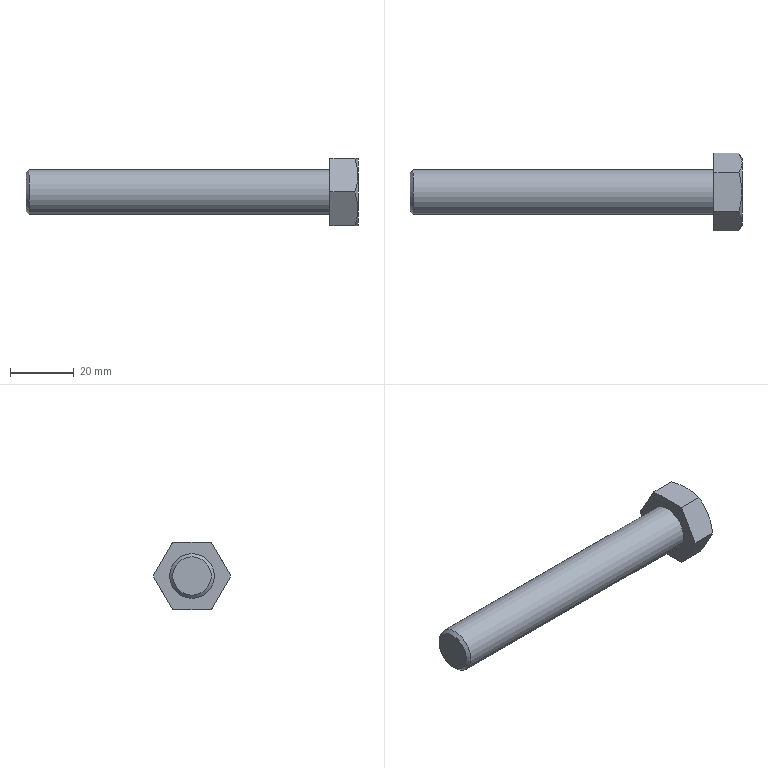Part | STEP file | 8901-M14 (bolt M14×95) | 1 solid | 12 faces | box 103.8 x 24.249 x 21 mm | volume 17952 mm3 | plane 9 | cone 2 | cylinder 1 | commonest cylinder face diameters 14 x1
STEP:
#1=CARTESIAN_POINT('',(0.,0.,0.));
#2=DIRECTION('',(0.,0.,1.));
#3=DIRECTION('',(1.,0.,0.));
#4=AXIS2_PLACEMENT_3D('',#1,#2,#3);
#5=CARTESIAN_POINT('',(1501.5,0.00003081,-188.));
#6=VERTEX_POINT('',#5);
#7=CARTESIAN_POINT('',(1501.5,0.00003081,-195.));
#8=DIRECTION('',(1.,0.,0.));
#9=DIRECTION('',(0.,0.,1.));
#10=AXIS2_PLACEMENT_3D('',#7,#8,#9);
#11=CIRCLE('',#10,7.);
#12=CARTESIAN_POINT('',(1501.5,0.00003081,-195.));
#13=DIRECTION('',(1.,0.,0.));
#14=DIRECTION('',(0.,0.,1.));
#15=AXIS2_PLACEMENT_3D('',#12,#13,#14);
#16=CONICAL_SURFACE('',#15,7.,0.7854);
#17=CARTESIAN_POINT('',(0.,0.));
#18=DIRECTION('',(1.,0.));
#19=VECTOR('',#18,1.);
#20=LINE('',#17,#19);
#21=(GEOMETRIC_REPRESENTATION_CONTEXT(2)PARAMETRIC_REPRESENTATION_CONTEXT()REPRESENTATION_CONTEXT('',''));
#22=DEFINITIONAL_REPRESENTATION('',(#20),#21);
#23=PCURVE('',#16,#22);
#24=CARTESIAN_POINT('',(1595.5,0.00003081,-195.));
#25=DIRECTION('',(-1.,0.,0.));
#26=DIRECTION('',(0.,0.,-1.));
#27=AXIS2_PLACEMENT_3D('',#24,#25,#26);
#28=CYLINDRICAL_SURFACE('',#27,7.);
#29=CARTESIAN_POINT('',(9.425,94.));
#30=DIRECTION('',(-1.,0.));
#31=VECTOR('',#30,1.);
#32=LINE('',#29,#31);
#33=(GEOMETRIC_REPRESENTATION_CONTEXT(2)PARAMETRIC_REPRESENTATION_CONTEXT()REPRESENTATION_CONTEXT('',''));
#34=DEFINITIONAL_REPRESENTATION('',(#32),#33);
#35=PCURVE('',#28,#34);
#36=SURFACE_CURVE('',#11,(#23,#35),.PCURVE_S1.);
#37=EDGE_CURVE('',#6,#6,#36,.T.);
#38=ORIENTED_EDGE('',*,*,#37,.F.);
#39=CARTESIAN_POINT('',(1500.5,0.00003081,-189.));
#40=VERTEX_POINT('',#39);
#41=CARTESIAN_POINT('',(1500.5,0.00003081,-189.));
#42=CARTESIAN_POINT('',(1501.5,0.00003081,-188.));
#43=B_SPLINE_CURVE_WITH_KNOTS('',1,(#41,#42),.UNSPECIFIED.,.F.,.F.,(2,2),(-1.414,0.),.PIECEWISE_BEZIER_KNOTS.);
#44=CARTESIAN_POINT('',(0.,0.));
#45=DIRECTION('',(0.,1.));
#46=VECTOR('',#45,1.);
#47=LINE('',#44,#46);
#48=(GEOMETRIC_REPRESENTATION_CONTEXT(2)PARAMETRIC_REPRESENTATION_CONTEXT()REPRESENTATION_CONTEXT('',''));
#49=DEFINITIONAL_REPRESENTATION('',(#47),#48);
#50=PCURVE('',#16,#49);
#51=CARTESIAN_POINT('',(6.283,0.));
#52=DIRECTION('',(0.,1.));
#53=VECTOR('',#52,1.);
#54=LINE('',#51,#53);
#55=(GEOMETRIC_REPRESENTATION_CONTEXT(2)PARAMETRIC_REPRESENTATION_CONTEXT()REPRESENTATION_CONTEXT('',''));
#56=DEFINITIONAL_REPRESENTATION('',(#54),#55);
#57=PCURVE('',#16,#56);
#58=SEAM_CURVE('',#43,(#50,#57),.PCURVE_S1.);
#59=EDGE_CURVE('',#40,#6,#58,.T.);
#60=ORIENTED_EDGE('',*,*,#59,.F.);
#61=CARTESIAN_POINT('',(1500.5,0.00003081,-195.));
#62=DIRECTION('',(-1.,0.,0.));
#63=DIRECTION('',(0.,0.,1.));
#64=AXIS2_PLACEMENT_3D('',#61,#62,#63);
#65=CIRCLE('',#64,6.);
#66=CARTESIAN_POINT('',(6.283,-1.));
#67=DIRECTION('',(-1.,0.));
#68=VECTOR('',#67,1.);
#69=LINE('',#66,#68);
#70=(GEOMETRIC_REPRESENTATION_CONTEXT(2)PARAMETRIC_REPRESENTATION_CONTEXT()REPRESENTATION_CONTEXT('',''));
#71=DEFINITIONAL_REPRESENTATION('',(#69),#70);
#72=PCURVE('',#16,#71);
#73=CARTESIAN_POINT('',(1500.5,0.00003081,-195.));
#74=DIRECTION('',(-1.,0.,0.));
#75=DIRECTION('',(0.,0.,-1.));
#76=AXIS2_PLACEMENT_3D('',#73,#74,#75);
#77=PLANE('',#76);
#78=CARTESIAN_POINT('',(0.,0.));
#79=DIRECTION('',(-1.,0.));
#80=AXIS2_PLACEMENT_2D('',#78,#79);
#81=CIRCLE('',#80,6.);
#82=(GEOMETRIC_REPRESENTATION_CONTEXT(2)PARAMETRIC_REPRESENTATION_CONTEXT()REPRESENTATION_CONTEXT('',''));
#83=DEFINITIONAL_REPRESENTATION('',(#81),#82);
#84=PCURVE('',#77,#83);
#85=SURFACE_CURVE('',#65,(#72,#84),.PCURVE_S1.);
#86=EDGE_CURVE('',#40,#40,#85,.T.);
#87=ORIENTED_EDGE('',*,*,#86,.F.);
#88=ORIENTED_EDGE('',*,*,#59,.T.);
#89=EDGE_LOOP('',(#38,#60,#87,#88));
#90=FACE_BOUND('',#89,.T.);
#91=ADVANCED_FACE('',(#90),#16,.T.);
#92=ORIENTED_EDGE('',*,*,#86,.T.);
#93=EDGE_LOOP('',(#92));
#94=FACE_BOUND('',#93,.T.);
#95=ADVANCED_FACE('',(#94),#77,.T.);
#96=CARTESIAN_POINT('',(1604.3,0.00003081,-205.395));
#97=VERTEX_POINT('',#96);
#98=CARTESIAN_POINT('',(1604.3,0.00003081,-195.));
#99=DIRECTION('',(1.,0.,0.));
#100=DIRECTION('',(0.,0.,-1.));
#101=AXIS2_PLACEMENT_3D('',#98,#99,#100);
#102=CIRCLE('',#101,10.395);
#103=CARTESIAN_POINT('',(1604.3,0.00003081,-195.));
#104=DIRECTION('',(1.,0.,0.));
#105=DIRECTION('',(0.,0.,1.));
#106=AXIS2_PLACEMENT_3D('',#103,#104,#105);
#107=PLANE('',#106);
#108=CARTESIAN_POINT('',(0.,0.));
#109=DIRECTION('',(-1.,0.));
#110=AXIS2_PLACEMENT_2D('',#108,#109);
#111=CIRCLE('',#110,10.395);
#112=(GEOMETRIC_REPRESENTATION_CONTEXT(2)PARAMETRIC_REPRESENTATION_CONTEXT()REPRESENTATION_CONTEXT('',''));
#113=DEFINITIONAL_REPRESENTATION('',(#111),#112);
#114=PCURVE('',#107,#113);
#115=CARTESIAN_POINT('',(1610.302,0.00003081,-195.));
#116=DIRECTION('',(-1.,0.,0.));
#117=DIRECTION('',(0.,0.,-1.));
#118=AXIS2_PLACEMENT_3D('',#115,#116,#117);
#119=CONICAL_SURFACE('',#118,0.,1.047);
#120=CARTESIAN_POINT('',(6.283,6.002));
#121=DIRECTION('',(-1.,0.));
#122=VECTOR('',#121,1.);
#123=LINE('',#120,#122);
#124=(GEOMETRIC_REPRESENTATION_CONTEXT(2)PARAMETRIC_REPRESENTATION_CONTEXT()REPRESENTATION_CONTEXT('',''));
#125=DEFINITIONAL_REPRESENTATION('',(#123),#124);
#126=PCURVE('',#119,#125);
#127=SURFACE_CURVE('',#102,(#114,#126),.PCURVE_S1.);
#128=EDGE_CURVE('',#97,#97,#127,.T.);
#129=ORIENTED_EDGE('',*,*,#128,.T.);
#130=EDGE_LOOP('',(#129));
#131=FACE_BOUND('',#130,.T.);
#132=ADVANCED_FACE('',(#131),#107,.T.);
#133=ORIENTED_EDGE('',*,*,#128,.F.);
#134=CARTESIAN_POINT('',(1604.239,0.00003081,-205.5));
#135=VERTEX_POINT('',#134);
#136=CARTESIAN_POINT('',(1604.3,0.00003081,-205.395));
#137=CARTESIAN_POINT('',(1604.239,0.00003081,-205.5));
#138=B_SPLINE_CURVE_WITH_KNOTS('',1,(#136,#137),.UNSPECIFIED.,.F.,.F.,(2,2),(12.003,12.124),.PIECEWISE_BEZIER_KNOTS.);
#139=CARTESIAN_POINT('',(6.283,0.));
#140=DIRECTION('',(0.,1.));
#141=VECTOR('',#140,1.);
#142=LINE('',#139,#141);
#143=(GEOMETRIC_REPRESENTATION_CONTEXT(2)PARAMETRIC_REPRESENTATION_CONTEXT()REPRESENTATION_CONTEXT('',''));
#144=DEFINITIONAL_REPRESENTATION('',(#142),#143);
#145=PCURVE('',#119,#144);
#146=CARTESIAN_POINT('',(0.,0.));
#147=DIRECTION('',(0.,1.));
#148=VECTOR('',#147,1.);
#149=LINE('',#146,#148);
#150=(GEOMETRIC_REPRESENTATION_CONTEXT(2)PARAMETRIC_REPRESENTATION_CONTEXT()REPRESENTATION_CONTEXT('',''));
#151=DEFINITIONAL_REPRESENTATION('',(#149),#150);
#152=PCURVE('',#119,#151);
#153=SEAM_CURVE('',#138,(#145,#152),.PCURVE_S1.);
#154=EDGE_CURVE('',#97,#135,#153,.T.);
#155=ORIENTED_EDGE('',*,*,#154,.T.);
#156=CARTESIAN_POINT('',(1603.302,6.062,-205.5));
#157=VERTEX_POINT('',#156);
#158=CARTESIAN_POINT('',(1603.302,6.062,-205.5));
#159=CARTESIAN_POINT('',(1603.873,4.083,-205.5));
#160=CARTESIAN_POINT('',(1604.238,2.073,-205.5));
#161=CARTESIAN_POINT('',(1604.241,-2.05,-205.5));
#162=CARTESIAN_POINT('',(1603.874,-4.08,-205.5));
#163=CARTESIAN_POINT('',(1603.302,-6.062,-205.5));
#164=B_SPLINE_CURVE_WITH_KNOTS('',3,(#158,#159,#160,#161,#162,#163),.UNSPECIFIED.,.F.,.F.,(4,2,4),(0.,0.5,1.),.UNSPECIFIED.);
#165=CARTESIAN_POINT('',(5.76,7.));
#166=CARTESIAN_POINT('',(5.772,6.948));
#167=CARTESIAN_POINT('',(5.799,6.847));
#168=CARTESIAN_POINT('',(5.84,6.707));
#169=CARTESIAN_POINT('',(5.883,6.579));
#170=CARTESIAN_POINT('',(5.928,6.463));
#171=CARTESIAN_POINT('',(5.975,6.36));
#172=CARTESIAN_POINT('',(6.023,6.271));
#173=CARTESIAN_POINT('',(6.073,6.197));
#174=CARTESIAN_POINT('',(6.124,6.138));
#175=CARTESIAN_POINT('',(6.176,6.095));
#176=CARTESIAN_POINT('',(6.229,6.068));
#177=CARTESIAN_POINT('',(6.282,6.059));
#178=CARTESIAN_POINT('',(6.336,6.068));
#179=CARTESIAN_POINT('',(6.389,6.093));
#180=CARTESIAN_POINT('',(6.441,6.136));
#181=CARTESIAN_POINT('',(6.492,6.195));
#182=CARTESIAN_POINT('',(6.542,6.269));
#183=CARTESIAN_POINT('',(6.591,6.358));
#184=CARTESIAN_POINT('',(6.638,6.461));
#185=CARTESIAN_POINT('',(6.683,6.578));
#186=CARTESIAN_POINT('',(6.726,6.707));
#187=CARTESIAN_POINT('',(6.768,6.847));
#188=CARTESIAN_POINT('',(6.794,6.948));
#189=CARTESIAN_POINT('',(6.807,7.));
#190=B_SPLINE_CURVE_WITH_KNOTS('',3,(#165,#166,#167,#168,#169,#170,#171,#172,#173,#174,#175,#176,#177,#178,#179,#180,#181,#182,#183,#184,#185,#186,#187,#188,#189),.UNSPECIFIED.,.F.,.F.,(4,1,1,1,1,1,1,1,1,1,1,1,1,1,1,1,1,1,1,1,1,1,4),(0.,0.04545,0.09091,0.1364,0.1818,0.2273,0.2727,0.3182,0.3636,0.4091,0.4545,0.5,0.5455,0.5909,0.6364,0.6818,0.7273,0.7727,0.8182,0.8636,0.9091,0.9545,1.),.QUASI_UNIFORM_KNOTS.);
#191=(GEOMETRIC_REPRESENTATION_CONTEXT(2)PARAMETRIC_REPRESENTATION_CONTEXT()REPRESENTATION_CONTEXT('',''));
#192=DEFINITIONAL_REPRESENTATION('',(#190),#191);
#193=PCURVE('',#119,#192);
#194=CARTESIAN_POINT('',(1599.9,0.00003081,-205.5));
#195=DIRECTION('',(0.,0.,-1.));
#196=DIRECTION('',(0.,-1.,0.));
#197=AXIS2_PLACEMENT_3D('',#194,#195,#196);
#198=PLANE('',#197);
#199=CARTESIAN_POINT('',(-6.062,-3.402));
#200=CARTESIAN_POINT('',(-4.082,-3.973));
#201=CARTESIAN_POINT('',(-2.073,-4.338));
#202=CARTESIAN_POINT('',(2.05,-4.341));
#203=CARTESIAN_POINT('',(4.08,-3.974));
#204=CARTESIAN_POINT('',(6.062,-3.402));
#205=B_SPLINE_CURVE_WITH_KNOTS('',3,(#199,#200,#201,#202,#203,#204),.UNSPECIFIED.,.F.,.F.,(4,2,4),(0.,0.5,1.),.UNSPECIFIED.);
#206=(GEOMETRIC_REPRESENTATION_CONTEXT(2)PARAMETRIC_REPRESENTATION_CONTEXT()REPRESENTATION_CONTEXT('',''));
#207=DEFINITIONAL_REPRESENTATION('',(#205),#206);
#208=PCURVE('',#198,#207);
#209=SURFACE_CURVE('',#164,(#193,#208),.PCURVE_S1.);
#210=EDGE_CURVE('',#157,#135,#209,.T.);
#211=ORIENTED_EDGE('',*,*,#210,.F.);
#212=CARTESIAN_POINT('',(1603.302,12.124,-195.));
#213=VERTEX_POINT('',#212);
#214=CARTESIAN_POINT('',(1603.302,12.124,-195.));
#215=CARTESIAN_POINT('',(1603.873,11.135,-196.714));
#216=CARTESIAN_POINT('',(1604.238,10.13,-198.455));
#217=CARTESIAN_POINT('',(1604.241,8.068,-202.025));
#218=CARTESIAN_POINT('',(1603.874,7.053,-203.783));
#219=CARTESIAN_POINT('',(1603.302,6.062,-205.5));
#220=B_SPLINE_CURVE_WITH_KNOTS('',3,(#214,#215,#216,#217,#218,#219),.UNSPECIFIED.,.F.,.F.,(4,2,4),(0.,0.5,1.),.UNSPECIFIED.);
#221=CARTESIAN_POINT('',(4.712,7.));
#222=CARTESIAN_POINT('',(4.725,6.948));
#223=CARTESIAN_POINT('',(4.752,6.847));
#224=CARTESIAN_POINT('',(4.793,6.707));
#225=CARTESIAN_POINT('',(4.836,6.579));
#226=CARTESIAN_POINT('',(4.881,6.463));
#227=CARTESIAN_POINT('',(4.928,6.36));
#228=CARTESIAN_POINT('',(4.976,6.271));
#229=CARTESIAN_POINT('',(5.026,6.197));
#230=CARTESIAN_POINT('',(5.076,6.138));
#231=CARTESIAN_POINT('',(5.129,6.095));
#232=CARTESIAN_POINT('',(5.181,6.068));
#233=CARTESIAN_POINT('',(5.235,6.059));
#234=CARTESIAN_POINT('',(5.288,6.068));
#235=CARTESIAN_POINT('',(5.341,6.093));
#236=CARTESIAN_POINT('',(5.394,6.136));
#237=CARTESIAN_POINT('',(5.445,6.195));
#238=CARTESIAN_POINT('',(5.495,6.269));
#239=CARTESIAN_POINT('',(5.543,6.358));
#240=CARTESIAN_POINT('',(5.59,6.461));
#241=CARTESIAN_POINT('',(5.636,6.578));
#242=CARTESIAN_POINT('',(5.679,6.707));
#243=CARTESIAN_POINT('',(5.72,6.847));
#244=CARTESIAN_POINT('',(5.747,6.948));
#245=CARTESIAN_POINT('',(5.76,7.));
#246=B_SPLINE_CURVE_WITH_KNOTS('',3,(#221,#222,#223,#224,#225,#226,#227,#228,#229,#230,#231,#232,#233,#234,#235,#236,#237,#238,#239,#240,#241,#242,#243,#244,#245),.UNSPECIFIED.,.F.,.F.,(4,1,1,1,1,1,1,1,1,1,1,1,1,1,1,1,1,1,1,1,1,1,4),(0.,0.04545,0.09091,0.1364,0.1818,0.2273,0.2727,0.3182,0.3636,0.4091,0.4545,0.5,0.5455,0.5909,0.6364,0.6818,0.7273,0.7727,0.8182,0.8636,0.9091,0.9545,1.),.QUASI_UNIFORM_KNOTS.);
#247=(GEOMETRIC_REPRESENTATION_CONTEXT(2)PARAMETRIC_REPRESENTATION_CONTEXT()REPRESENTATION_CONTEXT('',''));
#248=DEFINITIONAL_REPRESENTATION('',(#246),#247);
#249=PCURVE('',#119,#248);
#250=CARTESIAN_POINT('',(1599.9,9.093,-200.25));
#251=DIRECTION('',(0.,0.866,-0.5));
#252=DIRECTION('',(0.,-0.5,-0.866));
#253=AXIS2_PLACEMENT_3D('',#250,#251,#252);
#254=PLANE('',#253);
#255=CARTESIAN_POINT('',(-6.062,-3.402));
#256=CARTESIAN_POINT('',(-4.082,-3.973));
#257=CARTESIAN_POINT('',(-2.073,-4.338));
#258=CARTESIAN_POINT('',(2.05,-4.341));
#259=CARTESIAN_POINT('',(4.08,-3.974));
#260=CARTESIAN_POINT('',(6.062,-3.402));
#261=B_SPLINE_CURVE_WITH_KNOTS('',3,(#255,#256,#257,#258,#259,#260),.UNSPECIFIED.,.F.,.F.,(4,2,4),(0.,0.5,1.),.UNSPECIFIED.);
#262=(GEOMETRIC_REPRESENTATION_CONTEXT(2)PARAMETRIC_REPRESENTATION_CONTEXT()REPRESENTATION_CONTEXT('',''));
#263=DEFINITIONAL_REPRESENTATION('',(#261),#262);
#264=PCURVE('',#254,#263);
#265=SURFACE_CURVE('',#220,(#249,#264),.PCURVE_S1.);
#266=EDGE_CURVE('',#213,#157,#265,.T.);
#267=ORIENTED_EDGE('',*,*,#266,.F.);
#268=CARTESIAN_POINT('',(1603.302,6.062,-184.5));
#269=VERTEX_POINT('',#268);
#270=CARTESIAN_POINT('',(1603.302,6.062,-184.5));
#271=CARTESIAN_POINT('',(1603.873,7.052,-186.214));
#272=CARTESIAN_POINT('',(1604.238,8.057,-187.955));
#273=CARTESIAN_POINT('',(1604.241,10.118,-191.525));
#274=CARTESIAN_POINT('',(1603.874,11.133,-193.283));
#275=CARTESIAN_POINT('',(1603.302,12.124,-195.));
#276=B_SPLINE_CURVE_WITH_KNOTS('',3,(#270,#271,#272,#273,#274,#275),.UNSPECIFIED.,.F.,.F.,(4,2,4),(0.,0.5,1.),.UNSPECIFIED.);
#277=CARTESIAN_POINT('',(3.665,7.));
#278=CARTESIAN_POINT('',(3.678,6.948));
#279=CARTESIAN_POINT('',(3.704,6.847));
#280=CARTESIAN_POINT('',(3.746,6.707));
#281=CARTESIAN_POINT('',(3.789,6.579));
#282=CARTESIAN_POINT('',(3.834,6.463));
#283=CARTESIAN_POINT('',(3.88,6.36));
#284=CARTESIAN_POINT('',(3.929,6.271));
#285=CARTESIAN_POINT('',(3.978,6.197));
#286=CARTESIAN_POINT('',(4.029,6.138));
#287=CARTESIAN_POINT('',(4.081,6.095));
#288=CARTESIAN_POINT('',(4.134,6.068));
#289=CARTESIAN_POINT('',(4.188,6.059));
#290=CARTESIAN_POINT('',(4.241,6.068));
#291=CARTESIAN_POINT('',(4.294,6.093));
#292=CARTESIAN_POINT('',(4.346,6.136));
#293=CARTESIAN_POINT('',(4.398,6.195));
#294=CARTESIAN_POINT('',(4.448,6.269));
#295=CARTESIAN_POINT('',(4.496,6.358));
#296=CARTESIAN_POINT('',(4.543,6.461));
#297=CARTESIAN_POINT('',(4.588,6.578));
#298=CARTESIAN_POINT('',(4.632,6.707));
#299=CARTESIAN_POINT('',(4.673,6.847));
#300=CARTESIAN_POINT('',(4.7,6.948));
#301=CARTESIAN_POINT('',(4.712,7.));
#302=B_SPLINE_CURVE_WITH_KNOTS('',3,(#277,#278,#279,#280,#281,#282,#283,#284,#285,#286,#287,#288,#289,#290,#291,#292,#293,#294,#295,#296,#297,#298,#299,#300,#301),.UNSPECIFIED.,.F.,.F.,(4,1,1,1,1,1,1,1,1,1,1,1,1,1,1,1,1,1,1,1,1,1,4),(0.,0.04545,0.09091,0.1364,0.1818,0.2273,0.2727,0.3182,0.3636,0.4091,0.4545,0.5,0.5455,0.5909,0.6364,0.6818,0.7273,0.7727,0.8182,0.8636,0.9091,0.9545,1.),.QUASI_UNIFORM_KNOTS.);
#303=(GEOMETRIC_REPRESENTATION_CONTEXT(2)PARAMETRIC_REPRESENTATION_CONTEXT()REPRESENTATION_CONTEXT('',''));
#304=DEFINITIONAL_REPRESENTATION('',(#302),#303);
#305=PCURVE('',#119,#304);
#306=CARTESIAN_POINT('',(1599.9,9.093,-189.75));
#307=DIRECTION('',(0.,0.866,0.5));
#308=DIRECTION('',(0.,0.5,-0.866));
#309=AXIS2_PLACEMENT_3D('',#306,#307,#308);
#310=PLANE('',#309);
#311=CARTESIAN_POINT('',(-6.062,-3.402));
#312=CARTESIAN_POINT('',(-4.082,-3.973));
#313=CARTESIAN_POINT('',(-2.073,-4.338));
#314=CARTESIAN_POINT('',(2.05,-4.341));
#315=CARTESIAN_POINT('',(4.08,-3.974));
#316=CARTESIAN_POINT('',(6.062,-3.402));
#317=B_SPLINE_CURVE_WITH_KNOTS('',3,(#311,#312,#313,#314,#315,#316),.UNSPECIFIED.,.F.,.F.,(4,2,4),(0.,0.5,1.),.UNSPECIFIED.);
#318=(GEOMETRIC_REPRESENTATION_CONTEXT(2)PARAMETRIC_REPRESENTATION_CONTEXT()REPRESENTATION_CONTEXT('',''));
#319=DEFINITIONAL_REPRESENTATION('',(#317),#318);
#320=PCURVE('',#310,#319);
#321=SURFACE_CURVE('',#276,(#305,#320),.PCURVE_S1.);
#322=EDGE_CURVE('',#269,#213,#321,.T.);
#323=ORIENTED_EDGE('',*,*,#322,.F.);
#324=CARTESIAN_POINT('',(1603.302,-6.062,-184.5));
#325=VERTEX_POINT('',#324);
#326=CARTESIAN_POINT('',(1603.302,-6.062,-184.5));
#327=CARTESIAN_POINT('',(1603.873,-4.082,-184.5));
#328=CARTESIAN_POINT('',(1604.238,-2.073,-184.5));
#329=CARTESIAN_POINT('',(1604.241,2.05,-184.5));
#330=CARTESIAN_POINT('',(1603.874,4.08,-184.5));
#331=CARTESIAN_POINT('',(1603.302,6.062,-184.5));
#332=B_SPLINE_CURVE_WITH_KNOTS('',3,(#326,#327,#328,#329,#330,#331),.UNSPECIFIED.,.F.,.F.,(4,2,4),(0.,0.5,1.),.UNSPECIFIED.);
#333=CARTESIAN_POINT('',(2.618,7.));
#334=CARTESIAN_POINT('',(2.631,6.948));
#335=CARTESIAN_POINT('',(2.657,6.847));
#336=CARTESIAN_POINT('',(2.698,6.707));
#337=CARTESIAN_POINT('',(2.742,6.579));
#338=CARTESIAN_POINT('',(2.787,6.463));
#339=CARTESIAN_POINT('',(2.833,6.36));
#340=CARTESIAN_POINT('',(2.881,6.271));
#341=CARTESIAN_POINT('',(2.931,6.197));
#342=CARTESIAN_POINT('',(2.982,6.138));
#343=CARTESIAN_POINT('',(3.034,6.095));
#344=CARTESIAN_POINT('',(3.087,6.068));
#345=CARTESIAN_POINT('',(3.14,6.059));
#346=CARTESIAN_POINT('',(3.194,6.068));
#347=CARTESIAN_POINT('',(3.247,6.093));
#348=CARTESIAN_POINT('',(3.299,6.136));
#349=CARTESIAN_POINT('',(3.351,6.195));
#350=CARTESIAN_POINT('',(3.401,6.269));
#351=CARTESIAN_POINT('',(3.449,6.358));
#352=CARTESIAN_POINT('',(3.496,6.461));
#353=CARTESIAN_POINT('',(3.541,6.578));
#354=CARTESIAN_POINT('',(3.584,6.707));
#355=CARTESIAN_POINT('',(3.626,6.847));
#356=CARTESIAN_POINT('',(3.652,6.948));
#357=CARTESIAN_POINT('',(3.665,7.));
#358=B_SPLINE_CURVE_WITH_KNOTS('',3,(#333,#334,#335,#336,#337,#338,#339,#340,#341,#342,#343,#344,#345,#346,#347,#348,#349,#350,#351,#352,#353,#354,#355,#356,#357),.UNSPECIFIED.,.F.,.F.,(4,1,1,1,1,1,1,1,1,1,1,1,1,1,1,1,1,1,1,1,1,1,4),(0.,0.04545,0.09091,0.1364,0.1818,0.2273,0.2727,0.3182,0.3636,0.4091,0.4545,0.5,0.5455,0.5909,0.6364,0.6818,0.7273,0.7727,0.8182,0.8636,0.9091,0.9545,1.),.QUASI_UNIFORM_KNOTS.);
#359=(GEOMETRIC_REPRESENTATION_CONTEXT(2)PARAMETRIC_REPRESENTATION_CONTEXT()REPRESENTATION_CONTEXT('',''));
#360=DEFINITIONAL_REPRESENTATION('',(#358),#359);
#361=PCURVE('',#119,#360);
#362=CARTESIAN_POINT('',(1599.9,0.00003081,-184.5));
#363=DIRECTION('',(0.,0.,1.));
#364=DIRECTION('',(0.,1.,0.));
#365=AXIS2_PLACEMENT_3D('',#362,#363,#364);
#366=PLANE('',#365);
#367=CARTESIAN_POINT('',(-6.062,-3.402));
#368=CARTESIAN_POINT('',(-4.082,-3.973));
#369=CARTESIAN_POINT('',(-2.073,-4.338));
#370=CARTESIAN_POINT('',(2.05,-4.341));
#371=CARTESIAN_POINT('',(4.08,-3.974));
#372=CARTESIAN_POINT('',(6.062,-3.402));
#373=B_SPLINE_CURVE_WITH_KNOTS('',3,(#367,#368,#369,#370,#371,#372),.UNSPECIFIED.,.F.,.F.,(4,2,4),(0.,0.5,1.),.UNSPECIFIED.);
#374=(GEOMETRIC_REPRESENTATION_CONTEXT(2)PARAMETRIC_REPRESENTATION_CONTEXT()REPRESENTATION_CONTEXT('',''));
#375=DEFINITIONAL_REPRESENTATION('',(#373),#374);
#376=PCURVE('',#366,#375);
#377=SURFACE_CURVE('',#332,(#361,#376),.PCURVE_S1.);
#378=EDGE_CURVE('',#325,#269,#377,.T.);
#379=ORIENTED_EDGE('',*,*,#378,.F.);
#380=CARTESIAN_POINT('',(1603.302,-12.124,-195.));
#381=VERTEX_POINT('',#380);
#382=CARTESIAN_POINT('',(1603.302,-12.124,-195.));
#383=CARTESIAN_POINT('',(1603.873,-11.134,-193.286));
#384=CARTESIAN_POINT('',(1604.238,-10.13,-191.545));
#385=CARTESIAN_POINT('',(1604.241,-8.068,-187.975));
#386=CARTESIAN_POINT('',(1603.874,-7.053,-186.217));
#387=CARTESIAN_POINT('',(1603.302,-6.062,-184.5));
#388=B_SPLINE_CURVE_WITH_KNOTS('',3,(#382,#383,#384,#385,#386,#387),.UNSPECIFIED.,.F.,.F.,(4,2,4),(0.,0.5,1.),.UNSPECIFIED.);
#389=CARTESIAN_POINT('',(1.571,7.));
#390=CARTESIAN_POINT('',(1.584,6.948));
#391=CARTESIAN_POINT('',(1.61,6.847));
#392=CARTESIAN_POINT('',(1.651,6.707));
#393=CARTESIAN_POINT('',(1.694,6.579));
#394=CARTESIAN_POINT('',(1.739,6.463));
#395=CARTESIAN_POINT('',(1.786,6.36));
#396=CARTESIAN_POINT('',(1.834,6.271));
#397=CARTESIAN_POINT('',(1.884,6.197));
#398=CARTESIAN_POINT('',(1.935,6.138));
#399=CARTESIAN_POINT('',(1.987,6.095));
#400=CARTESIAN_POINT('',(2.04,6.068));
#401=CARTESIAN_POINT('',(2.093,6.059));
#402=CARTESIAN_POINT('',(2.147,6.068));
#403=CARTESIAN_POINT('',(2.2,6.093));
#404=CARTESIAN_POINT('',(2.252,6.136));
#405=CARTESIAN_POINT('',(2.303,6.195));
#406=CARTESIAN_POINT('',(2.353,6.269));
#407=CARTESIAN_POINT('',(2.402,6.358));
#408=CARTESIAN_POINT('',(2.449,6.461));
#409=CARTESIAN_POINT('',(2.494,6.578));
#410=CARTESIAN_POINT('',(2.537,6.707));
#411=CARTESIAN_POINT('',(2.579,6.847));
#412=CARTESIAN_POINT('',(2.605,6.948));
#413=CARTESIAN_POINT('',(2.618,7.));
#414=B_SPLINE_CURVE_WITH_KNOTS('',3,(#389,#390,#391,#392,#393,#394,#395,#396,#397,#398,#399,#400,#401,#402,#403,#404,#405,#406,#407,#408,#409,#410,#411,#412,#413),.UNSPECIFIED.,.F.,.F.,(4,1,1,1,1,1,1,1,1,1,1,1,1,1,1,1,1,1,1,1,1,1,4),(0.,0.04545,0.09091,0.1364,0.1818,0.2273,0.2727,0.3182,0.3636,0.4091,0.4545,0.5,0.5455,0.5909,0.6364,0.6818,0.7273,0.7727,0.8182,0.8636,0.9091,0.9545,1.),.QUASI_UNIFORM_KNOTS.);
#415=(GEOMETRIC_REPRESENTATION_CONTEXT(2)PARAMETRIC_REPRESENTATION_CONTEXT()REPRESENTATION_CONTEXT('',''));
#416=DEFINITIONAL_REPRESENTATION('',(#414),#415);
#417=PCURVE('',#119,#416);
#418=CARTESIAN_POINT('',(1599.9,-9.093,-189.75));
#419=DIRECTION('',(0.,-0.866,0.5));
#420=DIRECTION('',(0.,0.5,0.866));
#421=AXIS2_PLACEMENT_3D('',#418,#419,#420);
#422=PLANE('',#421);
#423=CARTESIAN_POINT('',(-6.062,-3.402));
#424=CARTESIAN_POINT('',(-4.082,-3.973));
#425=CARTESIAN_POINT('',(-2.073,-4.338));
#426=CARTESIAN_POINT('',(2.05,-4.341));
#427=CARTESIAN_POINT('',(4.08,-3.974));
#428=CARTESIAN_POINT('',(6.062,-3.402));
#429=B_SPLINE_CURVE_WITH_KNOTS('',3,(#423,#424,#425,#426,#427,#428),.UNSPECIFIED.,.F.,.F.,(4,2,4),(0.,0.5,1.),.UNSPECIFIED.);
#430=(GEOMETRIC_REPRESENTATION_CONTEXT(2)PARAMETRIC_REPRESENTATION_CONTEXT()REPRESENTATION_CONTEXT('',''));
#431=DEFINITIONAL_REPRESENTATION('',(#429),#430);
#432=PCURVE('',#422,#431);
#433=SURFACE_CURVE('',#388,(#417,#432),.PCURVE_S1.);
#434=EDGE_CURVE('',#381,#325,#433,.T.);
#435=ORIENTED_EDGE('',*,*,#434,.F.);
#436=CARTESIAN_POINT('',(1603.302,-6.062,-205.5));
#437=VERTEX_POINT('',#436);
#438=CARTESIAN_POINT('',(1603.302,-6.062,-205.5));
#439=CARTESIAN_POINT('',(1603.873,-7.052,-203.786));
#440=CARTESIAN_POINT('',(1604.238,-8.057,-202.045));
#441=CARTESIAN_POINT('',(1604.241,-10.118,-198.475));
#442=CARTESIAN_POINT('',(1603.874,-11.133,-196.717));
#443=CARTESIAN_POINT('',(1603.302,-12.124,-195.));
#444=B_SPLINE_CURVE_WITH_KNOTS('',3,(#438,#439,#440,#441,#442,#443),.UNSPECIFIED.,.F.,.F.,(4,2,4),(0.,0.5,1.),.UNSPECIFIED.);
#445=CARTESIAN_POINT('',(0.5236,7.));
#446=CARTESIAN_POINT('',(0.5365,6.948));
#447=CARTESIAN_POINT('',(0.5628,6.847));
#448=CARTESIAN_POINT('',(0.6041,6.707));
#449=CARTESIAN_POINT('',(0.6472,6.579));
#450=CARTESIAN_POINT('',(0.6921,6.463));
#451=CARTESIAN_POINT('',(0.7388,6.36));
#452=CARTESIAN_POINT('',(0.787,6.271));
#453=CARTESIAN_POINT('',(0.8367,6.197));
#454=CARTESIAN_POINT('',(0.8877,6.138));
#455=CARTESIAN_POINT('',(0.9398,6.095));
#456=CARTESIAN_POINT('',(0.9926,6.068));
#457=CARTESIAN_POINT('',(1.046,6.059));
#458=CARTESIAN_POINT('',(1.1,6.068));
#459=CARTESIAN_POINT('',(1.153,6.093));
#460=CARTESIAN_POINT('',(1.205,6.136));
#461=CARTESIAN_POINT('',(1.256,6.195));
#462=CARTESIAN_POINT('',(1.306,6.269));
#463=CARTESIAN_POINT('',(1.355,6.358));
#464=CARTESIAN_POINT('',(1.402,6.461));
#465=CARTESIAN_POINT('',(1.447,6.578));
#466=CARTESIAN_POINT('',(1.49,6.707));
#467=CARTESIAN_POINT('',(1.532,6.847));
#468=CARTESIAN_POINT('',(1.558,6.948));
#469=CARTESIAN_POINT('',(1.571,7.));
#470=B_SPLINE_CURVE_WITH_KNOTS('',3,(#445,#446,#447,#448,#449,#450,#451,#452,#453,#454,#455,#456,#457,#458,#459,#460,#461,#462,#463,#464,#465,#466,#467,#468,#469),.UNSPECIFIED.,.F.,.F.,(4,1,1,1,1,1,1,1,1,1,1,1,1,1,1,1,1,1,1,1,1,1,4),(0.,0.04545,0.09091,0.1364,0.1818,0.2273,0.2727,0.3182,0.3636,0.4091,0.4545,0.5,0.5455,0.5909,0.6364,0.6818,0.7273,0.7727,0.8182,0.8636,0.9091,0.9545,1.),.QUASI_UNIFORM_KNOTS.);
#471=(GEOMETRIC_REPRESENTATION_CONTEXT(2)PARAMETRIC_REPRESENTATION_CONTEXT()REPRESENTATION_CONTEXT('',''));
#472=DEFINITIONAL_REPRESENTATION('',(#470),#471);
#473=PCURVE('',#119,#472);
#474=CARTESIAN_POINT('',(1599.9,-9.093,-200.25));
#475=DIRECTION('',(0.,-0.866,-0.5));
#476=DIRECTION('',(0.,-0.5,0.866));
#477=AXIS2_PLACEMENT_3D('',#474,#475,#476);
#478=PLANE('',#477);
#479=CARTESIAN_POINT('',(-6.062,-3.402));
#480=CARTESIAN_POINT('',(-4.082,-3.973));
#481=CARTESIAN_POINT('',(-2.073,-4.338));
#482=CARTESIAN_POINT('',(2.05,-4.341));
#483=CARTESIAN_POINT('',(4.08,-3.974));
#484=CARTESIAN_POINT('',(6.062,-3.402));
#485=B_SPLINE_CURVE_WITH_KNOTS('',3,(#479,#480,#481,#482,#483,#484),.UNSPECIFIED.,.F.,.F.,(4,2,4),(0.,0.5,1.),.UNSPECIFIED.);
#486=(GEOMETRIC_REPRESENTATION_CONTEXT(2)PARAMETRIC_REPRESENTATION_CONTEXT()REPRESENTATION_CONTEXT('',''));
#487=DEFINITIONAL_REPRESENTATION('',(#485),#486);
#488=PCURVE('',#478,#487);
#489=SURFACE_CURVE('',#444,(#473,#488),.PCURVE_S1.);
#490=EDGE_CURVE('',#437,#381,#489,.T.);
#491=ORIENTED_EDGE('',*,*,#490,.F.);
#492=CARTESIAN_POINT('',(1603.302,6.062,-205.5));
#493=CARTESIAN_POINT('',(1603.873,4.083,-205.5));
#494=CARTESIAN_POINT('',(1604.238,2.073,-205.5));
#495=CARTESIAN_POINT('',(1604.241,-2.05,-205.5));
#496=CARTESIAN_POINT('',(1603.874,-4.08,-205.5));
#497=CARTESIAN_POINT('',(1603.302,-6.062,-205.5));
#498=B_SPLINE_CURVE_WITH_KNOTS('',3,(#492,#493,#494,#495,#496,#497),.UNSPECIFIED.,.F.,.F.,(4,2,4),(0.,0.5,1.),.UNSPECIFIED.);
#499=CARTESIAN_POINT('',(-0.5236,7.));
#500=CARTESIAN_POINT('',(-0.5107,6.948));
#501=CARTESIAN_POINT('',(-0.4844,6.847));
#502=CARTESIAN_POINT('',(-0.4431,6.707));
#503=CARTESIAN_POINT('',(-0.4,6.579));
#504=CARTESIAN_POINT('',(-0.3551,6.463));
#505=CARTESIAN_POINT('',(-0.3084,6.36));
#506=CARTESIAN_POINT('',(-0.2602,6.271));
#507=CARTESIAN_POINT('',(-0.2105,6.197));
#508=CARTESIAN_POINT('',(-0.1595,6.138));
#509=CARTESIAN_POINT('',(-0.1074,6.095));
#510=CARTESIAN_POINT('',(-0.05458,6.068));
#511=CARTESIAN_POINT('',(-0.001113,6.059));
#512=CARTESIAN_POINT('',(0.0524,6.068));
#513=CARTESIAN_POINT('',(0.1054,6.093));
#514=CARTESIAN_POINT('',(0.1577,6.136));
#515=CARTESIAN_POINT('',(0.2089,6.195));
#516=CARTESIAN_POINT('',(0.2589,6.269));
#517=CARTESIAN_POINT('',(0.3075,6.358));
#518=CARTESIAN_POINT('',(0.3544,6.461));
#519=CARTESIAN_POINT('',(0.3996,6.578));
#520=CARTESIAN_POINT('',(0.4429,6.707));
#521=CARTESIAN_POINT('',(0.4844,6.847));
#522=CARTESIAN_POINT('',(0.5107,6.948));
#523=CARTESIAN_POINT('',(0.5236,7.));
#524=B_SPLINE_CURVE_WITH_KNOTS('',3,(#499,#500,#501,#502,#503,#504,#505,#506,#507,#508,#509,#510,#511,#512,#513,#514,#515,#516,#517,#518,#519,#520,#521,#522,#523),.UNSPECIFIED.,.F.,.F.,(4,1,1,1,1,1,1,1,1,1,1,1,1,1,1,1,1,1,1,1,1,1,4),(0.,0.04545,0.09091,0.1364,0.1818,0.2273,0.2727,0.3182,0.3636,0.4091,0.4545,0.5,0.5455,0.5909,0.6364,0.6818,0.7273,0.7727,0.8182,0.8636,0.9091,0.9545,1.),.QUASI_UNIFORM_KNOTS.);
#525=(GEOMETRIC_REPRESENTATION_CONTEXT(2)PARAMETRIC_REPRESENTATION_CONTEXT()REPRESENTATION_CONTEXT('',''));
#526=DEFINITIONAL_REPRESENTATION('',(#524),#525);
#527=PCURVE('',#119,#526);
#528=CARTESIAN_POINT('',(-6.062,-3.402));
#529=CARTESIAN_POINT('',(-4.082,-3.973));
#530=CARTESIAN_POINT('',(-2.073,-4.338));
#531=CARTESIAN_POINT('',(2.05,-4.341));
#532=CARTESIAN_POINT('',(4.08,-3.974));
#533=CARTESIAN_POINT('',(6.062,-3.402));
#534=B_SPLINE_CURVE_WITH_KNOTS('',3,(#528,#529,#530,#531,#532,#533),.UNSPECIFIED.,.F.,.F.,(4,2,4),(0.,0.5,1.),.UNSPECIFIED.);
#535=(GEOMETRIC_REPRESENTATION_CONTEXT(2)PARAMETRIC_REPRESENTATION_CONTEXT()REPRESENTATION_CONTEXT('',''));
#536=DEFINITIONAL_REPRESENTATION('',(#534),#535);
#537=PCURVE('',#198,#536);
#538=SURFACE_CURVE('',#498,(#527,#537),.PCURVE_S1.);
#539=EDGE_CURVE('',#135,#437,#538,.T.);
#540=ORIENTED_EDGE('',*,*,#539,.F.);
#541=ORIENTED_EDGE('',*,*,#154,.F.);
#542=EDGE_LOOP('',(#133,#155,#211,#267,#323,#379,#435,#491,#540,#541));
#543=FACE_BOUND('',#542,.T.);
#544=ADVANCED_FACE('',(#543),#119,.T.);
#545=CARTESIAN_POINT('',(1595.5,-12.124,-195.));
#546=VERTEX_POINT('',#545);
#547=CARTESIAN_POINT('',(1595.5,-6.062,-205.5));
#548=VERTEX_POINT('',#547);
#549=CARTESIAN_POINT('',(1595.5,-12.124,-195.));
#550=DIRECTION('',(0.,0.5,-0.866));
#551=VECTOR('',#550,1.);
#552=LINE('',#549,#551);
#553=CARTESIAN_POINT('',(1595.5,0.00003081,-195.));
#554=DIRECTION('',(-1.,0.,0.));
#555=DIRECTION('',(0.,0.,-1.));
#556=AXIS2_PLACEMENT_3D('',#553,#554,#555);
#557=PLANE('',#556);
#558=CARTESIAN_POINT('',(0.,12.124));
#559=DIRECTION('',(0.866,-0.5));
#560=VECTOR('',#559,1.);
#561=LINE('',#558,#560);
#562=(GEOMETRIC_REPRESENTATION_CONTEXT(2)PARAMETRIC_REPRESENTATION_CONTEXT()REPRESENTATION_CONTEXT('',''));
#563=DEFINITIONAL_REPRESENTATION('',(#561),#562);
#564=PCURVE('',#557,#563);
#565=CARTESIAN_POINT('',(6.062,4.4));
#566=DIRECTION('',(-1.,0.));
#567=VECTOR('',#566,1.);
#568=LINE('',#565,#567);
#569=(GEOMETRIC_REPRESENTATION_CONTEXT(2)PARAMETRIC_REPRESENTATION_CONTEXT()REPRESENTATION_CONTEXT('',''));
#570=DEFINITIONAL_REPRESENTATION('',(#568),#569);
#571=PCURVE('',#478,#570);
#572=SURFACE_CURVE('',#552,(#564,#571),.PCURVE_S1.);
#573=EDGE_CURVE('',#546,#548,#572,.T.);
#574=ORIENTED_EDGE('',*,*,#573,.F.);
#575=CARTESIAN_POINT('',(1595.5,-6.062,-184.5));
#576=VERTEX_POINT('',#575);
#577=CARTESIAN_POINT('',(1595.5,-6.062,-184.5));
#578=DIRECTION('',(0.,-0.5,-0.866));
#579=VECTOR('',#578,1.);
#580=LINE('',#577,#579);
#581=CARTESIAN_POINT('',(-10.5,6.062));
#582=DIRECTION('',(0.866,0.5));
#583=VECTOR('',#582,1.);
#584=LINE('',#581,#583);
#585=(GEOMETRIC_REPRESENTATION_CONTEXT(2)PARAMETRIC_REPRESENTATION_CONTEXT()REPRESENTATION_CONTEXT('',''));
#586=DEFINITIONAL_REPRESENTATION('',(#584),#585);
#587=PCURVE('',#557,#586);
#588=CARTESIAN_POINT('',(6.062,4.4));
#589=DIRECTION('',(-1.,0.));
#590=VECTOR('',#589,1.);
#591=LINE('',#588,#590);
#592=(GEOMETRIC_REPRESENTATION_CONTEXT(2)PARAMETRIC_REPRESENTATION_CONTEXT()REPRESENTATION_CONTEXT('',''));
#593=DEFINITIONAL_REPRESENTATION('',(#591),#592);
#594=PCURVE('',#422,#593);
#595=SURFACE_CURVE('',#580,(#587,#594),.PCURVE_S1.);
#596=EDGE_CURVE('',#576,#546,#595,.T.);
#597=ORIENTED_EDGE('',*,*,#596,.F.);
#598=CARTESIAN_POINT('',(1595.5,6.062,-184.5));
#599=VERTEX_POINT('',#598);
#600=CARTESIAN_POINT('',(1595.5,6.062,-184.5));
#601=DIRECTION('',(0.,-1.,0.));
#602=VECTOR('',#601,1.);
#603=LINE('',#600,#602);
#604=CARTESIAN_POINT('',(-10.5,-6.062));
#605=DIRECTION('',(0.,1.));
#606=VECTOR('',#605,1.);
#607=LINE('',#604,#606);
#608=(GEOMETRIC_REPRESENTATION_CONTEXT(2)PARAMETRIC_REPRESENTATION_CONTEXT()REPRESENTATION_CONTEXT('',''));
#609=DEFINITIONAL_REPRESENTATION('',(#607),#608);
#610=PCURVE('',#557,#609);
#611=CARTESIAN_POINT('',(6.062,4.4));
#612=DIRECTION('',(-1.,0.));
#613=VECTOR('',#612,1.);
#614=LINE('',#611,#613);
#615=(GEOMETRIC_REPRESENTATION_CONTEXT(2)PARAMETRIC_REPRESENTATION_CONTEXT()REPRESENTATION_CONTEXT('',''));
#616=DEFINITIONAL_REPRESENTATION('',(#614),#615);
#617=PCURVE('',#366,#616);
#618=SURFACE_CURVE('',#603,(#610,#617),.PCURVE_S1.);
#619=EDGE_CURVE('',#599,#576,#618,.T.);
#620=ORIENTED_EDGE('',*,*,#619,.F.);
#621=CARTESIAN_POINT('',(1595.5,12.124,-195.));
#622=VERTEX_POINT('',#621);
#623=CARTESIAN_POINT('',(1595.5,12.124,-195.));
#624=DIRECTION('',(0.,-0.5,0.866));
#625=VECTOR('',#624,1.);
#626=LINE('',#623,#625);
#627=CARTESIAN_POINT('',(0.,-12.124));
#628=DIRECTION('',(-0.866,0.5));
#629=VECTOR('',#628,1.);
#630=LINE('',#627,#629);
#631=(GEOMETRIC_REPRESENTATION_CONTEXT(2)PARAMETRIC_REPRESENTATION_CONTEXT()REPRESENTATION_CONTEXT('',''));
#632=DEFINITIONAL_REPRESENTATION('',(#630),#631);
#633=PCURVE('',#557,#632);
#634=CARTESIAN_POINT('',(6.062,4.4));
#635=DIRECTION('',(-1.,0.));
#636=VECTOR('',#635,1.);
#637=LINE('',#634,#636);
#638=(GEOMETRIC_REPRESENTATION_CONTEXT(2)PARAMETRIC_REPRESENTATION_CONTEXT()REPRESENTATION_CONTEXT('',''));
#639=DEFINITIONAL_REPRESENTATION('',(#637),#638);
#640=PCURVE('',#310,#639);
#641=SURFACE_CURVE('',#626,(#633,#640),.PCURVE_S1.);
#642=EDGE_CURVE('',#622,#599,#641,.T.);
#643=ORIENTED_EDGE('',*,*,#642,.F.);
#644=CARTESIAN_POINT('',(1595.5,6.062,-205.5));
#645=VERTEX_POINT('',#644);
#646=CARTESIAN_POINT('',(1595.5,6.062,-205.5));
#647=DIRECTION('',(0.,0.5,0.866));
#648=VECTOR('',#647,1.);
#649=LINE('',#646,#648);
#650=CARTESIAN_POINT('',(10.5,-6.062));
#651=DIRECTION('',(-0.866,-0.5));
#652=VECTOR('',#651,1.);
#653=LINE('',#650,#652);
#654=(GEOMETRIC_REPRESENTATION_CONTEXT(2)PARAMETRIC_REPRESENTATION_CONTEXT()REPRESENTATION_CONTEXT('',''));
#655=DEFINITIONAL_REPRESENTATION('',(#653),#654);
#656=PCURVE('',#557,#655);
#657=CARTESIAN_POINT('',(6.062,4.4));
#658=DIRECTION('',(-1.,0.));
#659=VECTOR('',#658,1.);
#660=LINE('',#657,#659);
#661=(GEOMETRIC_REPRESENTATION_CONTEXT(2)PARAMETRIC_REPRESENTATION_CONTEXT()REPRESENTATION_CONTEXT('',''));
#662=DEFINITIONAL_REPRESENTATION('',(#660),#661);
#663=PCURVE('',#254,#662);
#664=SURFACE_CURVE('',#649,(#656,#663),.PCURVE_S1.);
#665=EDGE_CURVE('',#645,#622,#664,.T.);
#666=ORIENTED_EDGE('',*,*,#665,.F.);
#667=CARTESIAN_POINT('',(1595.5,-6.062,-205.5));
#668=DIRECTION('',(0.,1.,0.));
#669=VECTOR('',#668,1.);
#670=LINE('',#667,#669);
#671=CARTESIAN_POINT('',(10.5,6.062));
#672=DIRECTION('',(0.,-1.));
#673=VECTOR('',#672,1.);
#674=LINE('',#671,#673);
#675=(GEOMETRIC_REPRESENTATION_CONTEXT(2)PARAMETRIC_REPRESENTATION_CONTEXT()REPRESENTATION_CONTEXT('',''));
#676=DEFINITIONAL_REPRESENTATION('',(#674),#675);
#677=PCURVE('',#557,#676);
#678=CARTESIAN_POINT('',(6.062,4.4));
#679=DIRECTION('',(-1.,0.));
#680=VECTOR('',#679,1.);
#681=LINE('',#678,#680);
#682=(GEOMETRIC_REPRESENTATION_CONTEXT(2)PARAMETRIC_REPRESENTATION_CONTEXT()REPRESENTATION_CONTEXT('',''));
#683=DEFINITIONAL_REPRESENTATION('',(#681),#682);
#684=PCURVE('',#198,#683);
#685=SURFACE_CURVE('',#670,(#677,#684),.PCURVE_S1.);
#686=EDGE_CURVE('',#548,#645,#685,.T.);
#687=ORIENTED_EDGE('',*,*,#686,.F.);
#688=EDGE_LOOP('',(#574,#597,#620,#643,#666,#687));
#689=FACE_BOUND('',#688,.T.);
#690=CARTESIAN_POINT('',(1595.5,0.00003081,-188.));
#691=VERTEX_POINT('',#690);
#692=CARTESIAN_POINT('',(1595.5,0.00003081,-195.));
#693=DIRECTION('',(-1.,0.,0.));
#694=DIRECTION('',(0.,0.,1.));
#695=AXIS2_PLACEMENT_3D('',#692,#693,#694);
#696=CIRCLE('',#695,7.);
#697=CARTESIAN_POINT('',(0.,0.));
#698=DIRECTION('',(-1.,0.));
#699=AXIS2_PLACEMENT_2D('',#697,#698);
#700=CIRCLE('',#699,7.);
#701=(GEOMETRIC_REPRESENTATION_CONTEXT(2)PARAMETRIC_REPRESENTATION_CONTEXT()REPRESENTATION_CONTEXT('',''));
#702=DEFINITIONAL_REPRESENTATION('',(#700),#701);
#703=PCURVE('',#557,#702);
#704=CARTESIAN_POINT('',(3.142,0.));
#705=DIRECTION('',(1.,0.));
#706=VECTOR('',#705,1.);
#707=LINE('',#704,#706);
#708=(GEOMETRIC_REPRESENTATION_CONTEXT(2)PARAMETRIC_REPRESENTATION_CONTEXT()REPRESENTATION_CONTEXT('',''));
#709=DEFINITIONAL_REPRESENTATION('',(#707),#708);
#710=PCURVE('',#28,#709);
#711=SURFACE_CURVE('',#696,(#703,#710),.PCURVE_S1.);
#712=EDGE_CURVE('',#691,#691,#711,.T.);
#713=ORIENTED_EDGE('',*,*,#712,.F.);
#714=EDGE_LOOP('',(#713));
#715=FACE_BOUND('',#714,.T.);
#716=ADVANCED_FACE('',(#689,#715),#557,.T.);
#717=CARTESIAN_POINT('',(1595.5,-6.062,-205.5));
#718=DIRECTION('',(1.,0.,0.));
#719=VECTOR('',#718,1.);
#720=LINE('',#717,#719);
#721=CARTESIAN_POINT('',(-6.062,4.4));
#722=DIRECTION('',(0.,-1.));
#723=VECTOR('',#722,1.);
#724=LINE('',#721,#723);
#725=(GEOMETRIC_REPRESENTATION_CONTEXT(2)PARAMETRIC_REPRESENTATION_CONTEXT()REPRESENTATION_CONTEXT('',''));
#726=DEFINITIONAL_REPRESENTATION('',(#724),#725);
#727=PCURVE('',#478,#726);
#728=CARTESIAN_POINT('',(6.062,4.4));
#729=DIRECTION('',(0.,-1.));
#730=VECTOR('',#729,1.);
#731=LINE('',#728,#730);
#732=(GEOMETRIC_REPRESENTATION_CONTEXT(2)PARAMETRIC_REPRESENTATION_CONTEXT()REPRESENTATION_CONTEXT('',''));
#733=DEFINITIONAL_REPRESENTATION('',(#731),#732);
#734=PCURVE('',#198,#733);
#735=SURFACE_CURVE('',#720,(#727,#734),.PCURVE_S1.);
#736=EDGE_CURVE('',#548,#437,#735,.T.);
#737=ORIENTED_EDGE('',*,*,#736,.T.);
#738=ORIENTED_EDGE('',*,*,#490,.T.);
#739=CARTESIAN_POINT('',(1595.5,-12.124,-195.));
#740=DIRECTION('',(1.,0.,0.));
#741=VECTOR('',#740,1.);
#742=LINE('',#739,#741);
#743=CARTESIAN_POINT('',(6.062,4.4));
#744=DIRECTION('',(0.,-1.));
#745=VECTOR('',#744,1.);
#746=LINE('',#743,#745);
#747=(GEOMETRIC_REPRESENTATION_CONTEXT(2)PARAMETRIC_REPRESENTATION_CONTEXT()REPRESENTATION_CONTEXT('',''));
#748=DEFINITIONAL_REPRESENTATION('',(#746),#747);
#749=PCURVE('',#478,#748);
#750=CARTESIAN_POINT('',(-6.062,4.4));
#751=DIRECTION('',(0.,-1.));
#752=VECTOR('',#751,1.);
#753=LINE('',#750,#752);
#754=(GEOMETRIC_REPRESENTATION_CONTEXT(2)PARAMETRIC_REPRESENTATION_CONTEXT()REPRESENTATION_CONTEXT('',''));
#755=DEFINITIONAL_REPRESENTATION('',(#753),#754);
#756=PCURVE('',#422,#755);
#757=SURFACE_CURVE('',#742,(#749,#756),.PCURVE_S1.);
#758=EDGE_CURVE('',#546,#381,#757,.T.);
#759=ORIENTED_EDGE('',*,*,#758,.F.);
#760=ORIENTED_EDGE('',*,*,#573,.T.);
#761=EDGE_LOOP('',(#737,#738,#759,#760));
#762=FACE_BOUND('',#761,.T.);
#763=ADVANCED_FACE('',(#762),#478,.T.);
#764=CARTESIAN_POINT('',(1595.5,6.062,-205.5));
#765=DIRECTION('',(1.,0.,0.));
#766=VECTOR('',#765,1.);
#767=LINE('',#764,#766);
#768=CARTESIAN_POINT('',(-6.062,4.4));
#769=DIRECTION('',(0.,-1.));
#770=VECTOR('',#769,1.);
#771=LINE('',#768,#770);
#772=(GEOMETRIC_REPRESENTATION_CONTEXT(2)PARAMETRIC_REPRESENTATION_CONTEXT()REPRESENTATION_CONTEXT('',''));
#773=DEFINITIONAL_REPRESENTATION('',(#771),#772);
#774=PCURVE('',#198,#773);
#775=CARTESIAN_POINT('',(6.062,4.4));
#776=DIRECTION('',(0.,-1.));
#777=VECTOR('',#776,1.);
#778=LINE('',#775,#777);
#779=(GEOMETRIC_REPRESENTATION_CONTEXT(2)PARAMETRIC_REPRESENTATION_CONTEXT()REPRESENTATION_CONTEXT('',''));
#780=DEFINITIONAL_REPRESENTATION('',(#778),#779);
#781=PCURVE('',#254,#780);
#782=SURFACE_CURVE('',#767,(#774,#781),.PCURVE_S1.);
#783=EDGE_CURVE('',#645,#157,#782,.T.);
#784=ORIENTED_EDGE('',*,*,#783,.T.);
#785=ORIENTED_EDGE('',*,*,#210,.T.);
#786=ORIENTED_EDGE('',*,*,#539,.T.);
#787=ORIENTED_EDGE('',*,*,#736,.F.);
#788=ORIENTED_EDGE('',*,*,#686,.T.);
#789=EDGE_LOOP('',(#784,#785,#786,#787,#788));
#790=FACE_BOUND('',#789,.T.);
#791=ADVANCED_FACE('',(#790),#198,.T.);
#792=CARTESIAN_POINT('',(1595.5,12.124,-195.));
#793=DIRECTION('',(1.,0.,0.));
#794=VECTOR('',#793,1.);
#795=LINE('',#792,#794);
#796=CARTESIAN_POINT('',(-6.062,4.4));
#797=DIRECTION('',(0.,-1.));
#798=VECTOR('',#797,1.);
#799=LINE('',#796,#798);
#800=(GEOMETRIC_REPRESENTATION_CONTEXT(2)PARAMETRIC_REPRESENTATION_CONTEXT()REPRESENTATION_CONTEXT('',''));
#801=DEFINITIONAL_REPRESENTATION('',(#799),#800);
#802=PCURVE('',#254,#801);
#803=CARTESIAN_POINT('',(6.062,4.4));
#804=DIRECTION('',(0.,-1.));
#805=VECTOR('',#804,1.);
#806=LINE('',#803,#805);
#807=(GEOMETRIC_REPRESENTATION_CONTEXT(2)PARAMETRIC_REPRESENTATION_CONTEXT()REPRESENTATION_CONTEXT('',''));
#808=DEFINITIONAL_REPRESENTATION('',(#806),#807);
#809=PCURVE('',#310,#808);
#810=SURFACE_CURVE('',#795,(#802,#809),.PCURVE_S1.);
#811=EDGE_CURVE('',#622,#213,#810,.T.);
#812=ORIENTED_EDGE('',*,*,#811,.T.);
#813=ORIENTED_EDGE('',*,*,#266,.T.);
#814=ORIENTED_EDGE('',*,*,#783,.F.);
#815=ORIENTED_EDGE('',*,*,#665,.T.);
#816=EDGE_LOOP('',(#812,#813,#814,#815));
#817=FACE_BOUND('',#816,.T.);
#818=ADVANCED_FACE('',(#817),#254,.T.);
#819=CARTESIAN_POINT('',(1595.5,6.062,-184.5));
#820=DIRECTION('',(1.,0.,0.));
#821=VECTOR('',#820,1.);
#822=LINE('',#819,#821);
#823=CARTESIAN_POINT('',(-6.062,4.4));
#824=DIRECTION('',(0.,-1.));
#825=VECTOR('',#824,1.);
#826=LINE('',#823,#825);
#827=(GEOMETRIC_REPRESENTATION_CONTEXT(2)PARAMETRIC_REPRESENTATION_CONTEXT()REPRESENTATION_CONTEXT('',''));
#828=DEFINITIONAL_REPRESENTATION('',(#826),#827);
#829=PCURVE('',#310,#828);
#830=CARTESIAN_POINT('',(6.062,4.4));
#831=DIRECTION('',(0.,-1.));
#832=VECTOR('',#831,1.);
#833=LINE('',#830,#832);
#834=(GEOMETRIC_REPRESENTATION_CONTEXT(2)PARAMETRIC_REPRESENTATION_CONTEXT()REPRESENTATION_CONTEXT('',''));
#835=DEFINITIONAL_REPRESENTATION('',(#833),#834);
#836=PCURVE('',#366,#835);
#837=SURFACE_CURVE('',#822,(#829,#836),.PCURVE_S1.);
#838=EDGE_CURVE('',#599,#269,#837,.T.);
#839=ORIENTED_EDGE('',*,*,#838,.T.);
#840=ORIENTED_EDGE('',*,*,#322,.T.);
#841=ORIENTED_EDGE('',*,*,#811,.F.);
#842=ORIENTED_EDGE('',*,*,#642,.T.);
#843=EDGE_LOOP('',(#839,#840,#841,#842));
#844=FACE_BOUND('',#843,.T.);
#845=ADVANCED_FACE('',(#844),#310,.T.);
#846=CARTESIAN_POINT('',(1595.5,-6.062,-184.5));
#847=DIRECTION('',(1.,0.,0.));
#848=VECTOR('',#847,1.);
#849=LINE('',#846,#848);
#850=CARTESIAN_POINT('',(-6.062,4.4));
#851=DIRECTION('',(0.,-1.));
#852=VECTOR('',#851,1.);
#853=LINE('',#850,#852);
#854=(GEOMETRIC_REPRESENTATION_CONTEXT(2)PARAMETRIC_REPRESENTATION_CONTEXT()REPRESENTATION_CONTEXT('',''));
#855=DEFINITIONAL_REPRESENTATION('',(#853),#854);
#856=PCURVE('',#366,#855);
#857=CARTESIAN_POINT('',(6.062,4.4));
#858=DIRECTION('',(0.,-1.));
#859=VECTOR('',#858,1.);
#860=LINE('',#857,#859);
#861=(GEOMETRIC_REPRESENTATION_CONTEXT(2)PARAMETRIC_REPRESENTATION_CONTEXT()REPRESENTATION_CONTEXT('',''));
#862=DEFINITIONAL_REPRESENTATION('',(#860),#861);
#863=PCURVE('',#422,#862);
#864=SURFACE_CURVE('',#849,(#856,#863),.PCURVE_S1.);
#865=EDGE_CURVE('',#576,#325,#864,.T.);
#866=ORIENTED_EDGE('',*,*,#865,.T.);
#867=ORIENTED_EDGE('',*,*,#378,.T.);
#868=ORIENTED_EDGE('',*,*,#838,.F.);
#869=ORIENTED_EDGE('',*,*,#619,.T.);
#870=EDGE_LOOP('',(#866,#867,#868,#869));
#871=FACE_BOUND('',#870,.T.);
#872=ADVANCED_FACE('',(#871),#366,.T.);
#873=ORIENTED_EDGE('',*,*,#758,.T.);
#874=ORIENTED_EDGE('',*,*,#434,.T.);
#875=ORIENTED_EDGE('',*,*,#865,.F.);
#876=ORIENTED_EDGE('',*,*,#596,.T.);
#877=EDGE_LOOP('',(#873,#874,#875,#876));
#878=FACE_BOUND('',#877,.T.);
#879=ADVANCED_FACE('',(#878),#422,.T.);
#880=ORIENTED_EDGE('',*,*,#712,.T.);
#881=CARTESIAN_POINT('',(1595.5,0.00003081,-188.));
#882=CARTESIAN_POINT('',(1501.5,0.00003081,-188.));
#883=B_SPLINE_CURVE_WITH_KNOTS('',1,(#881,#882),.UNSPECIFIED.,.F.,.F.,(2,2),(0.,94.),.PIECEWISE_BEZIER_KNOTS.);
#884=CARTESIAN_POINT('',(9.425,0.));
#885=DIRECTION('',(0.,1.));
#886=VECTOR('',#885,1.);
#887=LINE('',#884,#886);
#888=(GEOMETRIC_REPRESENTATION_CONTEXT(2)PARAMETRIC_REPRESENTATION_CONTEXT()REPRESENTATION_CONTEXT('',''));
#889=DEFINITIONAL_REPRESENTATION('',(#887),#888);
#890=PCURVE('',#28,#889);
#891=CARTESIAN_POINT('',(3.142,0.));
#892=DIRECTION('',(0.,1.));
#893=VECTOR('',#892,1.);
#894=LINE('',#891,#893);
#895=(GEOMETRIC_REPRESENTATION_CONTEXT(2)PARAMETRIC_REPRESENTATION_CONTEXT()REPRESENTATION_CONTEXT('',''));
#896=DEFINITIONAL_REPRESENTATION('',(#894),#895);
#897=PCURVE('',#28,#896);
#898=SEAM_CURVE('',#883,(#890,#897),.PCURVE_S1.);
#899=EDGE_CURVE('',#691,#6,#898,.T.);
#900=ORIENTED_EDGE('',*,*,#899,.T.);
#901=ORIENTED_EDGE('',*,*,#37,.T.);
#902=ORIENTED_EDGE('',*,*,#899,.F.);
#903=EDGE_LOOP('',(#880,#900,#901,#902));
#904=FACE_BOUND('',#903,.T.);
#905=ADVANCED_FACE('',(#904),#28,.T.);
#906=CLOSED_SHELL('',(#91,#95,#132,#544,#716,#763,#791,#818,#845,#872,#879,#905));
#907=MANIFOLD_SOLID_BREP('',#906);
#908=(LENGTH_UNIT()NAMED_UNIT(*)SI_UNIT(.MILLI.,.METRE.));
#909=UNCERTAINTY_MEASURE_WITH_UNIT(LENGTH_MEASURE(0.001),#908,'','');
#910=(NAMED_UNIT(*)PLANE_ANGLE_UNIT()SI_UNIT($,.RADIAN.));
#911=(NAMED_UNIT(*)SI_UNIT($,.STERADIAN.)SOLID_ANGLE_UNIT());
#912=(GEOMETRIC_REPRESENTATION_CONTEXT(3)GLOBAL_UNCERTAINTY_ASSIGNED_CONTEXT((#909))GLOBAL_UNIT_ASSIGNED_CONTEXT((#908,#910,#911))REPRESENTATION_CONTEXT('',''));
#913=ADVANCED_BREP_SHAPE_REPRESENTATION('',(#4,#907),#912);